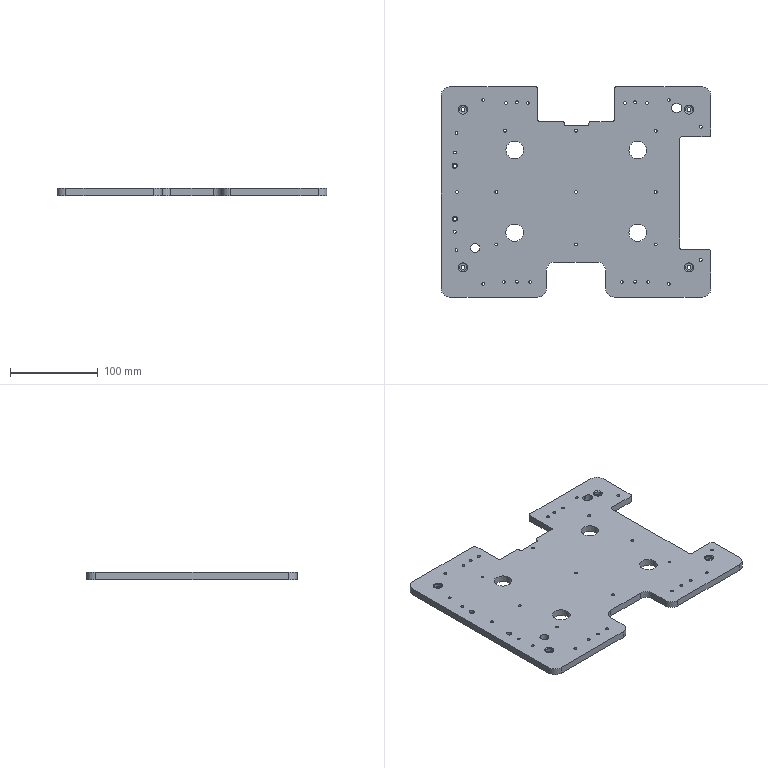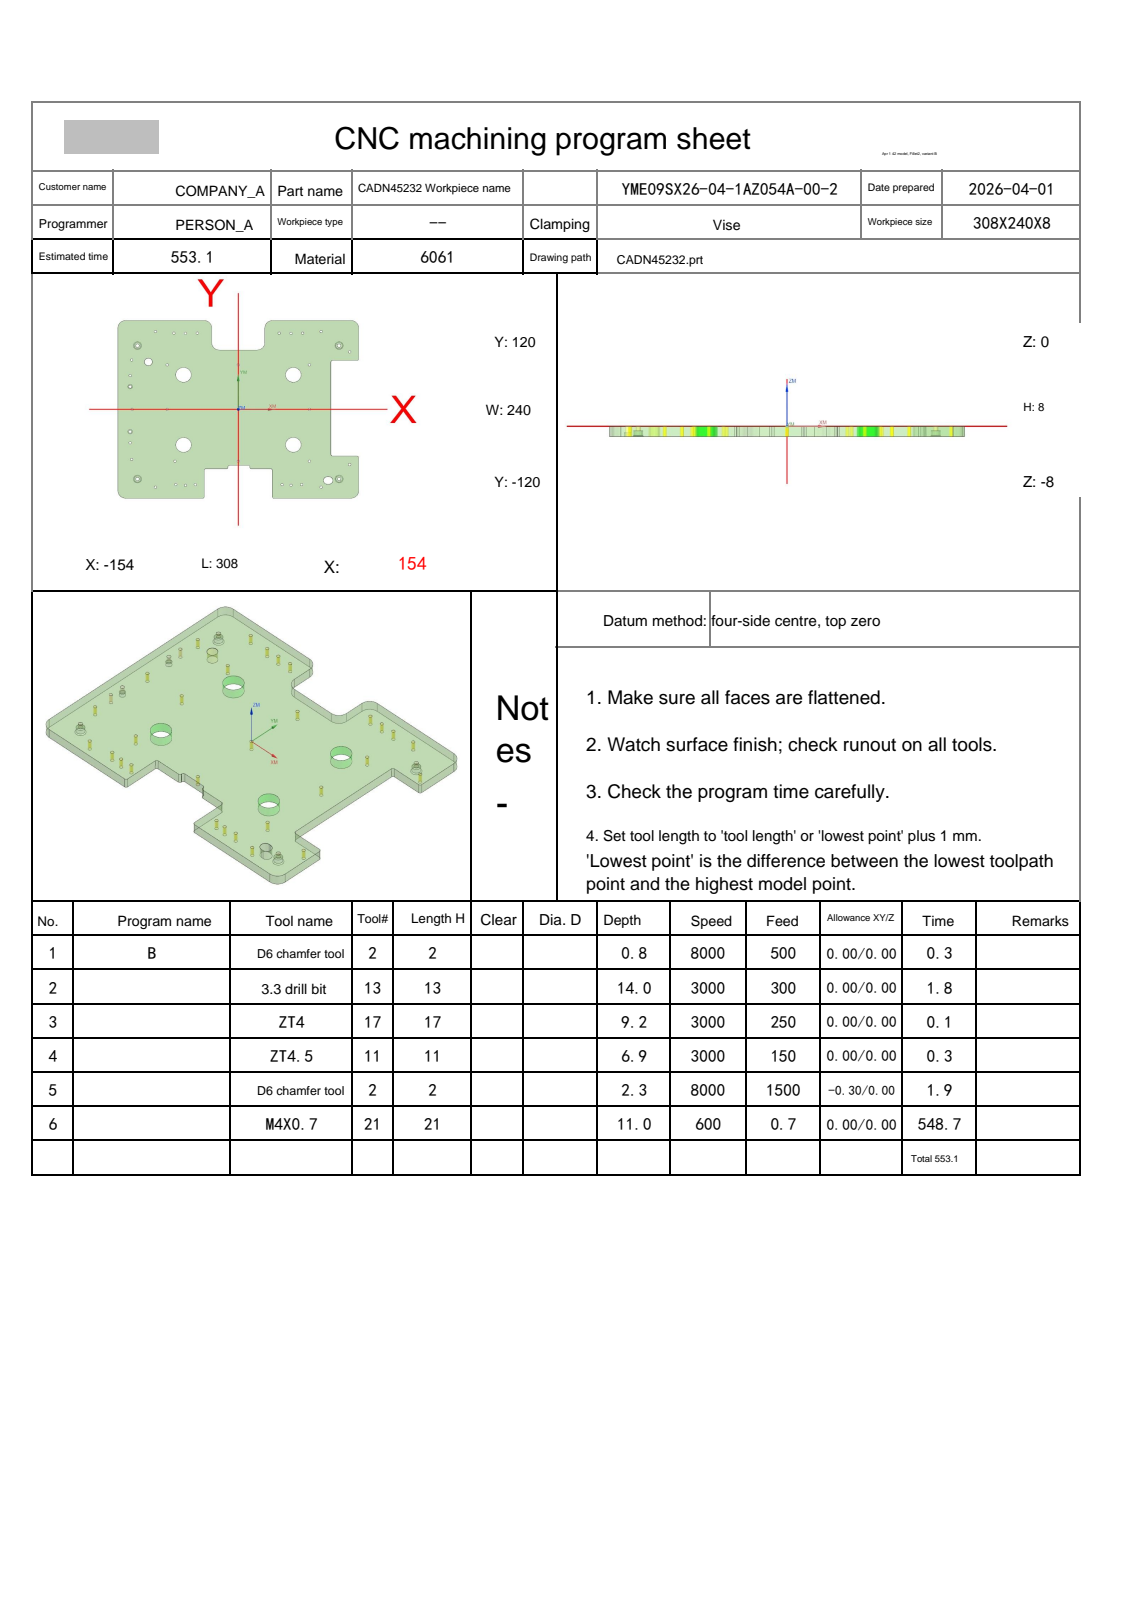NC program | NX | posted by the shop | part box 308 x 240 x 8 mm
Whole program:
%
O0001
(Machine time: 1056.89 MIN)
(===Total Tool:5===)
(T2=D6 chamfer tool   D=6.   R=0.   D-  H02 Z=-2.3  )
(T13=3.3 drill bit  D=3.3  DR_a=118 D-  H13 Z=-13.99)
(T17=ZT4    D=4.   DR_a=118 D-  H17 Z=-9.2  )
(T11=ZT4.5  D=4.5  DR_a=118 D-  H11 Z=-6.85 )
(T21=M4X0.7 D=3.3  DR_a=180 D-  H21 Z=-11.  )
G80 G90 G17 G49 G40
G91 G28 Z0
M01
N1 T02 M06
(D6 chamfer tool  D=6. R=0. H=02 ce=0.00 di=0.00)
G00 G90 G54 X142.5 Y-74.508 M03 S8000
G43 H02 Z20.
M08
G98 G81 X142.5 Y-74.508 Z-.8 R1. F500.
X129. Y-94.009
X106. Y-105.
X81. Y-101.6
X67.5 Y-102.5
X56. Y-101.6
X91. Y-70.
X70.458 Y-47.847
X91. Y0.0
X70.458 Y46.566
X91. Y60.
X142.5 Y77.5
X129. Y85.991
X106. Y105.
X82.35 Y102.765
X67.5 Y102.5
X52.35 Y102.765
X0.0 Y60.
Y0.0
Y-70.
X-70. Y-48.
X-81. Y-70.
X-55. Y-101.6
X-67.5 Y-102.5
X-80. Y-101.6
X-106. Y-105.
X-129. Y-94.009
X-136.5 Y-67.5
X-138.327 Y-45.083
Y-30.083
X-135.8 Y0.0
X-138.327 Y30.597
Y45.597
X-136.5 Y66.5
X-129. Y85.991
X-106. Y105.
X-82.35 Y102.765
X-67.5 Y102.5
X-52.35 Y102.765
X-91. Y60.
X-70.105 Y46.566
X-91. Y0.0
G80
G00 Z20.
G00 G90 X-115. Y63.991 M03 S8000
Z20.
G98 G82 X-115. Y63.991 Z-.8 R1. F500.
G80
G00 Z20.
G91 G28 Z0.0
M05
M09
G91 G28 Z0.0
M01
N2 T13 M06
(3.3 drill bit D=3.3 DR_a=118 H=13)
G00 G90 G54 X-52.35 Y102.765 M03 S3000
G43 H13 Z20.
M08
G98 G83 X-52.35 Y102.765 Z-13.991 R1. F300. Q2.
X-67.5 Y102.5
X-82.35 Y102.765
X-106. Y105.
X-136.5 Y66.5
X-138.327 Y45.597
X-91. Y60.
Y0.0
X-135.8
X-138.327 Y-45.083
X-136.5 Y-67.5
X-106. Y-105.
X-81. Y-70.
X-80. Y-101.6
X-67.5 Y-102.5
X-55. Y-101.6
X0.0 Y-70.
X56. Y-101.6
X67.5 Y-102.5
X81. Y-101.6
X106. Y-105.
X142.5 Y-74.508
X91. Y-70.
Y0.0
Y60.
X142.5 Y77.5
X106. Y105.
X82.35 Y102.765
X67.5 Y102.5
X52.35 Y102.765
X0.0 Y60.
Y0.0
G80
G00 Z20.
G91 G28 Z0.0
M05
M09
G91 G28 Z0.0
M01
N3 T17 M06
(ZT4 D=4. DR_a=118 H=17)
G00 G90 G54 X-138.327 Y-30.083 M03 S3000
G43 H17 Z20.
M08
G98 G83 X-138.327 Y-30.083 Z-9.202 R1. F250. Q2.
Y30.597
G80
G00 Z20.
G91 G28 Z0.0
M05
M09
G91 G28 Z0.0
M01
N4 T11 M06
(ZT4.5 D=4.5 DR_a=118 H=11)
G00 G90 G54 X-129. Y85.991 M03 S3000
G43 H11 Z20.
M08
G98 G83 X-129. Y85.991 Z-6.852 R1. F150. Q3.
Y-94.009
X129.
Y85.991
G80
G00 Z20.
G91 G28 Z0.0
M05
M09
G91 G28 Z0.0
M01
N5 T02 M06
(D6 chamfer tool  D=6. R=0. H=02 ce=-0.30 di=0.00)
G00 G90 G54 X-112.53 Y67.695 M03 S7000
G43 H02 Z20.
M08
Z2.5
G01 X-112.632 Y67.766 Z2.455 F1500.
X-112.915 Y67.93 Z2.336
X-113.323 Y68.12 Z2.172
X-113.748 Y68.268 Z2.008
X-114.186 Y68.372 Z1.844
X-114.632 Y68.432 Z1.681
X-115.082 Y68.447 Z1.517
X-115.531 Y68.416 Z1.353
X-115.974 Y68.34 Z1.189
X-116.408 Y68.219 Z1.025
X-116.827 Y68.055 Z.862
X-117.228 Y67.85 Z.698
X-117.606 Y67.606 Z.534
X-117.957 Y67.325 Z.37
X-118.278 Y67.009 Z.206
X-118.566 Y66.663 Z.042
X-118.817 Y66.29 Z-.121
X-119.03 Y65.893 Z-.285
X-119.201 Y65.477 Z-.449
X-119.33 Y65.045 Z-.613
X-119.414 Y64.603 Z-.777
X-119.453 Y64.155 Z-.94
Y63.991 Z-1.
G03 X-115. Y59.538 I4.453 J0.0
X-110.547 Y63.991 I0.0 J4.453
X-115. Y68.444 I-4.453 J0.0
X-119.453 Y63.991 I0.0 J-4.453
X-119.425 Y63.492 I4.453 J0.0
G01 Z1.5
G00 Z20.
X-65.349 Y38.577
Z2.5
G01 X-65.172 Y38.678 Z2.426
X-64.629 Y39.045 Z2.187
X-64.113 Y39.45 Z1.949
X-63.627 Y39.889 Z1.71
X-63.173 Y40.362 Z1.472
X-62.753 Y40.865 Z1.233
X-62.37 Y41.397 Z.994
X-62.025 Y41.954 Z.756
X-61.721 Y42.535 Z.517
X-61.458 Y43.135 Z.279
X-61.238 Y43.752 Z.04
X-61.061 Y44.384 Z-.198
X-60.93 Y45.026 Z-.437
X-60.845 Y45.676 Z-.675
X-60.805 Y46.33 Z-.914
Y46.566 Z-1.
G03 X-70.105 Y55.866 I-9.3 J0.0
X-79.405 Y46.566 I0.0 J-9.3
X-70.105 Y37.266 I9.3 J0.0
X-60.805 Y46.566 I0.0 J9.3
X-60.818 Y47.066 I-9.3 J0.0
G01 Z1.5
G00 Z20.
X-74.756 Y-40.01
Z2.5
G01 X-74.932 Y-40.112 Z2.426
X-75.476 Y-40.479 Z2.187
X-75.992 Y-40.883 Z1.949
X-76.478 Y-41.323 Z1.71
X-76.932 Y-41.796 Z1.472
X-77.351 Y-42.299 Z1.233
X-77.735 Y-42.831 Z.994
X-78.079 Y-43.388 Z.756
X-78.384 Y-43.969 Z.517
X-78.647 Y-44.569 Z.279
X-78.867 Y-45.186 Z.04
X-79.043 Y-45.818 Z-.198
X-79.175 Y-46.46 Z-.437
X-79.26 Y-47.11 Z-.675
X-79.3 Y-47.764 Z-.914
Y-48. Z-1.
G03 X-70. Y-57.3 I9.3 J0.0
X-60.7 Y-48. I0.0 J9.3
X-70. Y-38.7 I-9.3 J0.0
X-79.3 Y-48. I0.0 J-9.3
X-79.287 Y-48.5 I9.3 J0.0
G01 Z1.5
G00 Z20.
X-31.865 Y-80.779
Z2.5
G01 X-41.481 Z-1.
X-41.615 Y-80.787
G03 X-42.8 Y-82.076 I.109 J-1.289
G01 Y-82.099
Y-118.
G02 X-45.5 Y-120.7 I-2.7 J0.0
G01 X-144.
G02 X-154.7 Y-110. I0.0 J10.7
G01 Y110.
G02 X-144. Y120.7 I10.7 J0.0
G01 X-44.
G02 X-33.3 Y110. I0.0 J-10.7
G01 Y90.
G03 X-24. Y80.7 I9.3 J0.0
G01 X24.
G03 X33.3 Y90. I0.0 J9.3
G01 Y110.
G02 X44. Y120.7 I10.7 J0.0
G01 X144.
G02 X154.7 Y110. I0.0 J-10.7
G01 Y67.996
G02 X152. Y65.296 I-2.7 J0.0
G01 X120.473
X120.339 Y65.289
G03 X119.153 Y64. I.108 J-1.289
G01 Y63.977
Y-60.985
X119.161 Y-61.119
G03 X120.45 Y-62.304 I1.289 J.109
G01 X120.473
X152.
G02 X154.7 Y-65.004 I0.0 J-2.7
G01 Y-110.
G02 X144. Y-120.7 I-10.7 J0.0
G01 X45.5
G02 X42.8 Y-118. I0.0 J2.7
G01 Y-82.099
X42.793 Y-81.965
G03 X41.503 Y-80.779 I-1.289 J-.108
G01 X41.481
X16.792
X16.737 Y-80.778
X16.544 Y-80.767
X16.245 Y-80.73
X15.843 Y-80.616
X15.463 Y-80.44
X15.115 Y-80.208
X14.807 Y-79.926
X14.546 Y-79.599
X14.338 Y-79.235
X14.189 Y-78.844
X14.102 Y-78.435
X14.085 Y-78.125
X14.084 Y-78.07
Y-77.706
G03 X12.784 Y-76.406 I-1.3 J0.0
G01 X-11.216
G03 X-12.516 Y-77.706 I0.0 J-1.3
G01 Y-78.07
X-12.518 Y-78.125
X-12.528 Y-78.318
X-12.565 Y-78.617
X-12.68 Y-79.019
X-12.855 Y-79.399
X-13.087 Y-79.748
X-13.37 Y-80.056
X-13.697 Y-80.317
X-14.06 Y-80.525
X-14.451 Y-80.674
X-14.86 Y-80.761
X-15.17 Y-80.778
X-15.225 Y-80.779
X-41.481
X-41.615 Y-80.787
X-41.759 Y-80.804
X-41.952 Y-80.86
X-41.97 Y-80.868
Z1.5
G00 Z20.
X75.214 Y38.577
Z2.5
G01 X75.391 Y38.678 Z2.426
X75.934 Y39.045 Z2.187
X76.45 Y39.45 Z1.949
X76.936 Y39.889 Z1.71
X77.39 Y40.362 Z1.472
X77.81 Y40.865 Z1.233
X78.193 Y41.397 Z.994
X78.538 Y41.954 Z.756
X78.842 Y42.535 Z.517
X79.105 Y43.135 Z.279
X79.325 Y43.752 Z.04
X79.502 Y44.384 Z-.198
X79.633 Y45.026 Z-.437
X79.719 Y45.676 Z-.675
X79.758 Y46.33 Z-.914
Y46.566 Z-1.
G03 X70.458 Y55.866 I-9.3 J0.0
X61.158 Y46.566 I0.0 J-9.3
X70.458 Y37.266 I9.3 J0.0
X79.758 Y46.566 I0.0 J9.3
X79.745 Y47.066 I-9.3 J0.0
G01 Z1.5
G00 Z20.
X75.214 Y-55.836
Z2.5
G01 X75.391 Y-55.735 Z2.426
X75.934 Y-55.368 Z2.187
X76.45 Y-54.963 Z1.949
X76.936 Y-54.524 Z1.71
X77.39 Y-54.051 Z1.472
X77.81 Y-53.548 Z1.233
X78.193 Y-53.016 Z.994
X78.538 Y-52.459 Z.756
X78.842 Y-51.878 Z.517
X79.105 Y-51.278 Z.279
X79.325 Y-50.661 Z.04
X79.502 Y-50.029 Z-.198
X79.633 Y-49.387 Z-.437
X79.719 Y-48.737 Z-.675
X79.758 Y-48.083 Z-.914
Y-47.847 Z-1.
G03 X70.458 Y-38.547 I-9.3 J0.0
X61.158 Y-47.847 I0.0 J-9.3
X70.458 Y-57.147 I9.3 J0.0
X79.758 Y-47.847 I0.0 J9.3
X79.745 Y-47.347 I-9.3 J0.0
G01 Z1.5
G00 Z20.
G00 G90 X110.617 Y-93.357 M03 S7000
Z20.
Z2.5
G01 X110.538 Y-93.453 Z2.454 F1500.
X110.301 Y-93.811 Z2.298
X110.1 Y-94.19 Z2.142
X109.938 Y-94.588 Z1.986
X109.817 Y-94.999 Z1.83
X109.737 Y-95.421 Z1.674
X109.7 Y-95.848 Z1.518
Y-96.169 Z1.401
X109.737 Y-96.597 Z1.245
X109.817 Y-97.018 Z1.088
X109.938 Y-97.43 Z.932
X110.1 Y-97.827 Z.776
X110.301 Y-98.206 Z.62
X110.538 Y-98.564 Z.464
X110.809 Y-98.896 Z.308
X111.113 Y-99.199 Z.151
X111.445 Y-99.471 Z-.005
X111.802 Y-99.708 Z-.161
X112.182 Y-99.909 Z-.317
X112.579 Y-100.07 Z-.473
X112.99 Y-100.192 Z-.629
X113.412 Y-100.271 Z-.785
X113.839 Y-100.309 Z-.942
X114. Z-1.
X116.
G03 X120.3 Y-96.009 I0.0 J4.3
X116. Y-91.709 I-4.3 J0.0
G01 X114.
G03 X109.7 Y-96.009 I0.0 J-4.3
X114. Y-100.309 I4.3 J0.0
G01 X114.5
Z1.5
G00 Z20.
G00 G90 X-52.35 Y102.765 M03 S8000
Z20.
G98 G81 X-52.35 Y102.765 Z-2.2 R3. F500.
X-67.5 Y102.5
X-82.35 Y102.765
X-106. Y105.
X-136.5 Y66.5
X-138.327 Y45.597
X-91. Y60.
Y0.0
X-135.8
X-138.327 Y-45.083
X-136.5 Y-67.5
X-106. Y-105.
X-81. Y-70.
X-80. Y-101.6
X-67.5 Y-102.5
X-55. Y-101.6
X0.0 Y-70.
X56. Y-101.6
X67.5 Y-102.5
X81. Y-101.6
X106. Y-105.
X142.5 Y-74.508
X91. Y-70.
Y0.0
Y60.
X142.5 Y77.5
X106. Y105.
X82.35 Y102.765
X67.5 Y102.5
X52.35 Y102.765
X0.0 Y60.
Y0.0
G80
G00 Z20.
G00 G90 X-138.327 Y-30.083 M03 S8000
Z20.
G98 G81 X-138.327 Y-30.083 Z-2.3 R3. F500.
Y30.597
G80
G00 Z20.
G00 G90 X-129.018 Y86.541 M03 S8000
Z20.
Z-.5
G01 Z-1. F500.
X-129.05 Y87.491
G03 X-130.55 Y85.991 I0.0 J-1.5
X-129. Y84.441 I1.55 J0.0
X-127.45 Y85.991 I0.0 J1.55
X-129. Y87.541 I-1.55 J0.0
X-130.55 Y85.991 I0.0 J-1.55
X-129.05 Y84.491 I1.5 J0.0
G01 X-129.018 Y85.442
Z-.5
G00 Z20.
X-128.982 Y-94.558
Z-.5
G01 Z-1.
X-128.95 Y-95.509
G03 X-127.45 Y-94.009 I0.0 J1.5
X-129. Y-92.459 I-1.55 J0.0
X-130.55 Y-94.009 I0.0 J-1.55
X-129. Y-95.559 I1.55 J0.0
X-127.45 Y-94.009 I0.0 J1.55
X-128.95 Y-92.509 I-1.5 J0.0
G01 X-128.982 Y-93.459
Z-.5
G00 Z20.
X129.018 Y-94.558
Z-.5
G01 Z-1.
X129.05 Y-95.509
G03 X130.55 Y-94.009 I0.0 J1.5
X129. Y-92.459 I-1.55 J0.0
X127.45 Y-94.009 I0.0 J-1.55
X129. Y-95.559 I1.55 J0.0
X130.55 Y-94.009 I0.0 J1.55
X129.05 Y-92.509 I-1.5 J0.0
G01 X129.018 Y-93.459
Z-.5
G00 Z20.
Y85.442
Z-.5
G01 Z-1.
X129.05 Y84.491
G03 X130.55 Y85.991 I0.0 J1.5
X129. Y87.541 I-1.55 J0.0
X127.45 Y85.991 I0.0 J-1.55
X129. Y84.441 I1.55 J0.0
X130.55 Y85.991 I0.0 J1.55
X129.05 Y87.491 I-1.5 J0.0
G01 X129.018 Y86.541
Z-.5
G00 Z20.
G91 G28 Z0.0
M05
M09
G91 G28 Z0.0
M01
N6 T21 M06
(M4X0.7 D=3.3 DR_a=180 H=21)
G00 G90 G54 X-52.35 Y102.765 M03 S600
G43 H21 Z20.
M08
G95
G98 G84 X-52.35 Y102.765 Z-11. R1. F.7 Q4.
X-67.5 Y102.5
X-82.35 Y102.765
X-106. Y105.
X-136.5 Y66.5
X-138.327 Y45.597
X-91. Y60.
Y0.0
X-135.8
X-138.327 Y-45.083
X-136.5 Y-67.5
X-106. Y-105.
X-81. Y-70.
X-80. Y-101.6
X-67.5 Y-102.5
X-55. Y-101.6
X0.0 Y-70.
X56. Y-101.6
X67.5 Y-102.5
X81. Y-101.6
X106. Y-105.
X142.5 Y-74.508
X91. Y-70.
Y0.0
Y60.
X142.5 Y77.5
X106. Y105.
X82.35 Y102.765
X67.5 Y102.5
X52.35 Y102.765
X0.0 Y60.
Y0.0
G80
G94
G00 Z20.
M05
M09
G91 G28 Z0.0
G91 G28 Y0.0
M30
%